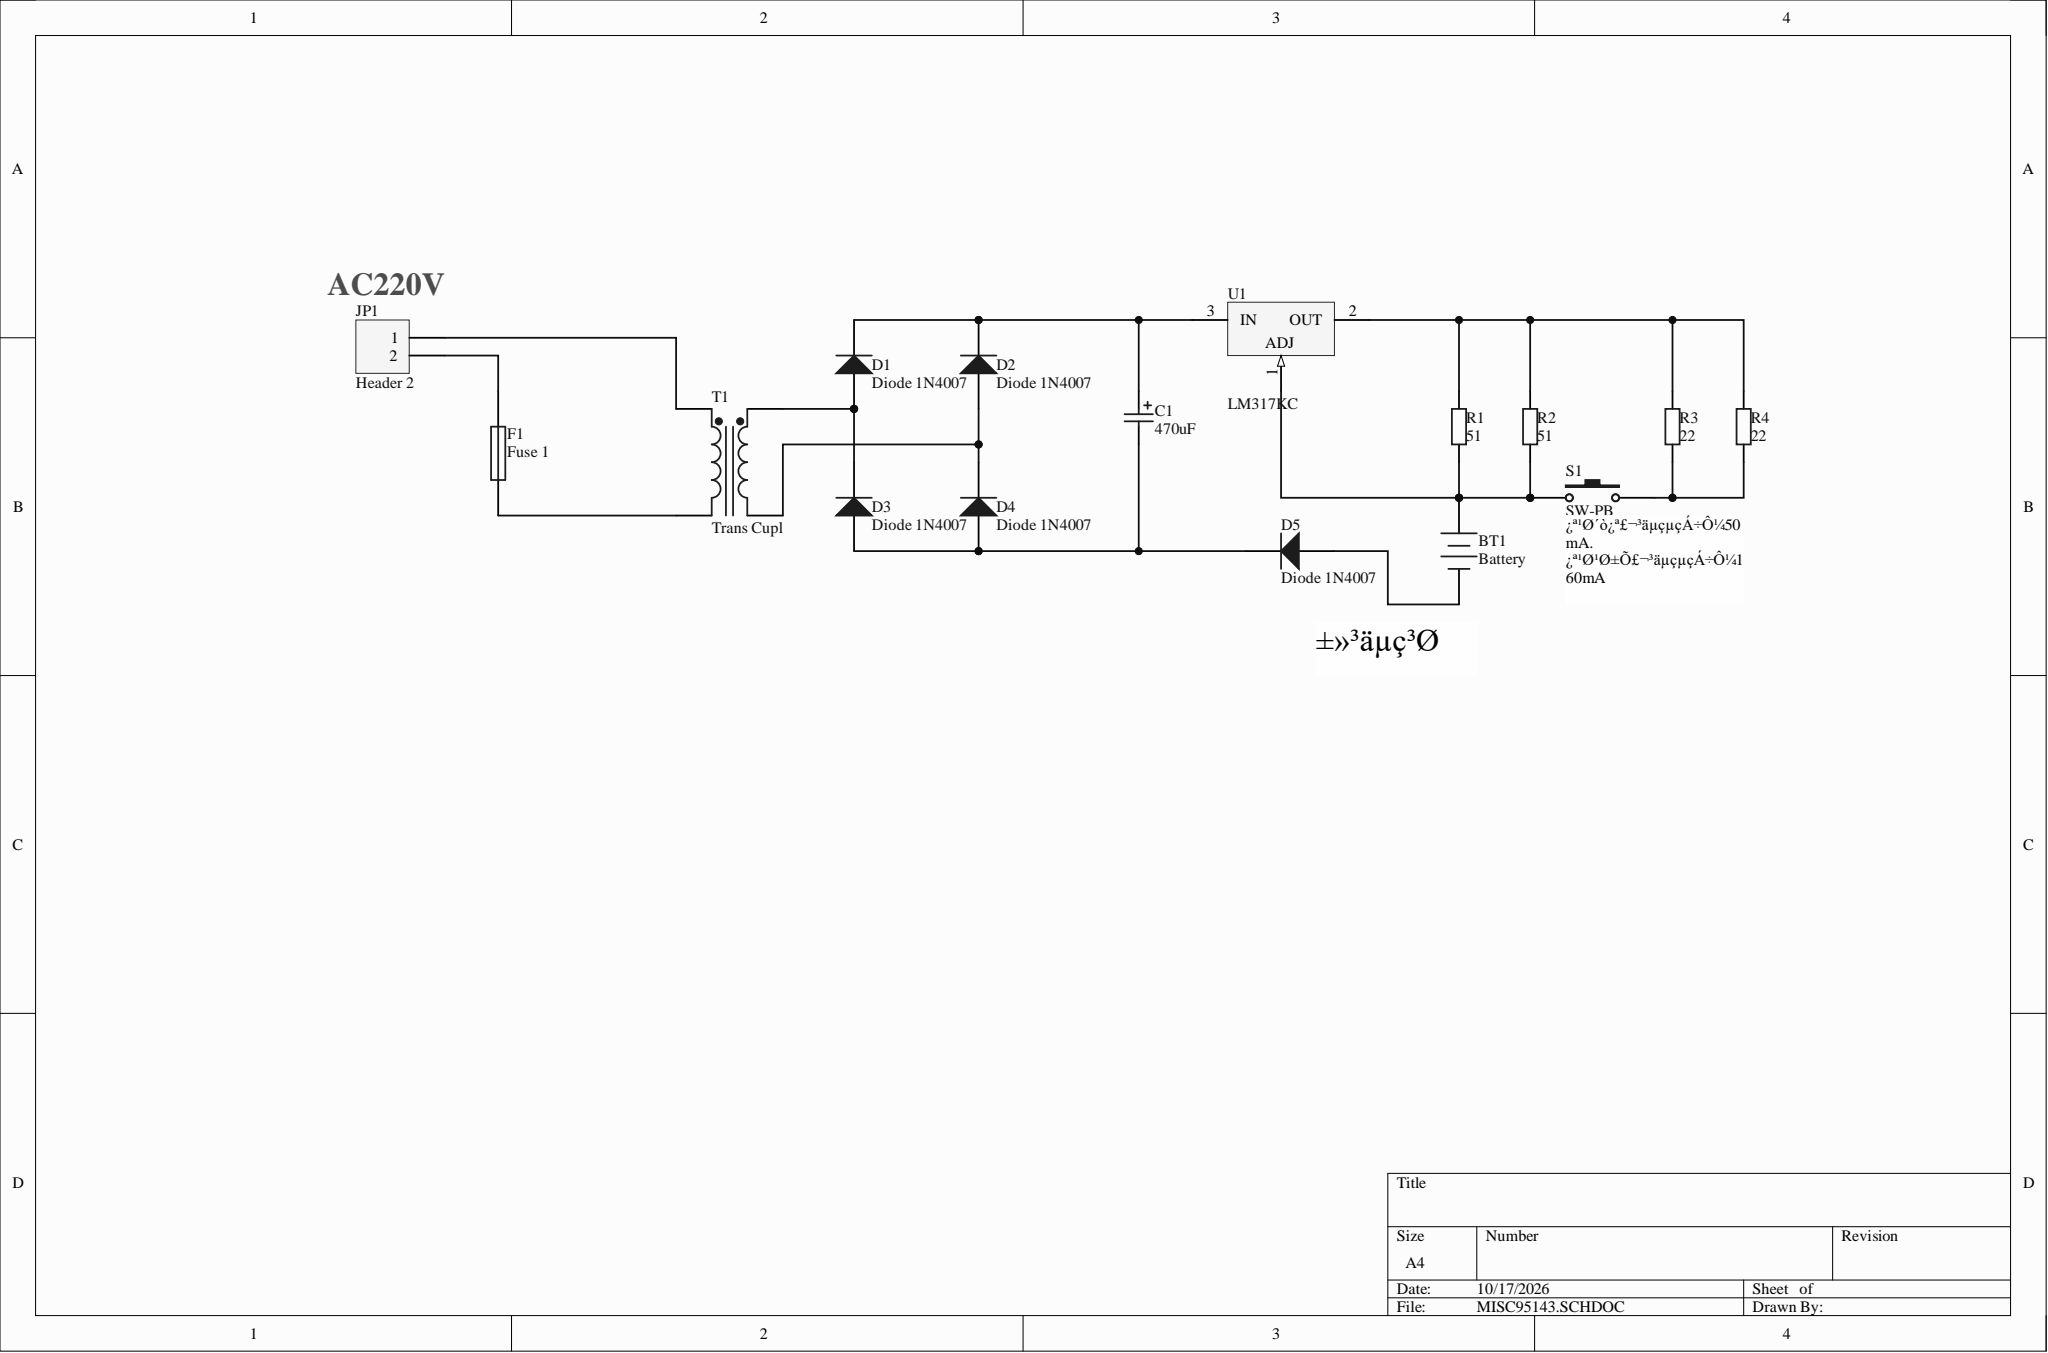Circuit board | Altium Designer | 16 parts | 11 nets
Bill of materials:
Comment,Description,Designator,Footprint,LibRef,Quantity
"Battery","Multicell Battery","BT1","BAT-2","Battery","1"
"Cap Pol1","Polarized Capacitor (Radial)","C1","RB7.6-15","Cap Pol1","1"
"Diode 1N4007","1 Amp General Purpose Rectifier","D1, D2, D3, D4, D5","DIO10.46-5.3x2.8","Diode 1N4007","5"
"Fuse 1","Fuse","F1","PIN-W2/E2.8","Fuse 1","1"
"Header 2","Header, 2-Pin","JP1","HDR1X2","Header 2","1"
"Res2","Resistor","R1, R2, R3, R4","AXIAL-0.4","Res2","4"
"SW-PB","Switch","S1","SPST-2","SW-PB","1"
"Trans Cupl","Transformer (Coupled Inductor Model)","T1","TRF_4","Trans Cupl","1"
"LM317KC","3-Terminal Adjustable Regulator","U1","KC03","LM317KC","1"
Netlist (Protel format):
[
BT1
BAT-2
Battery



]
[
C1
RB7.6-15
Cap Pol1



]
[
D1
DIO10.46-5.3x2.8
Diode 1N4007



]
[
D2
DIO10.46-5.3x2.8
Diode 1N4007



]
[
D3
DIO10.46-5.3x2.8
Diode 1N4007



]
[
D4
DIO10.46-5.3x2.8
Diode 1N4007



]
[
D5
DIO10.46-5.3x2.8
Diode 1N4007



]
[
F1
PIN-W2/E2.8
Fuse 1



]
[
JP1
HDR1X2
Header 2



]
[
R1
AXIAL-0.4
Res2



]
[
R2
AXIAL-0.4
Res2



]
[
R3
AXIAL-0.4
Res2



]
[
R4
AXIAL-0.4
Res2



]
[
S1
SPST-2
SW-PB



]
[
T1
TRF_4
Trans Cupl



]
[
U1
KC03
LM317KC



]
(
NetR3_1
R3-1
R4-1
S1-2
)
(
NetR1_2
R1-2
R2-2
R3-2
R4-2
U1-2
)
(
NetJP1_1
JP1-1
T1-1
)
(
NetF1_2
F1-2
JP1-2
)
(
NetF1_1
F1-1
T1-2
)
(
NetD2_1
D2-1
D4-2
T1-4
)
(
NetD1_1
D1-1
D3-2
T1-3
)
(
NetC1_2
C1-2
D3-1
D4-1
D5-2
)
(
NetC1_1
C1-1
D1-2
D2-2
U1-3
)
(
NetBT1_2
BT1-2
D5-1
)
(
NetBT1_1
BT1-1
R1-1
R2-1
S1-1
U1-1
)